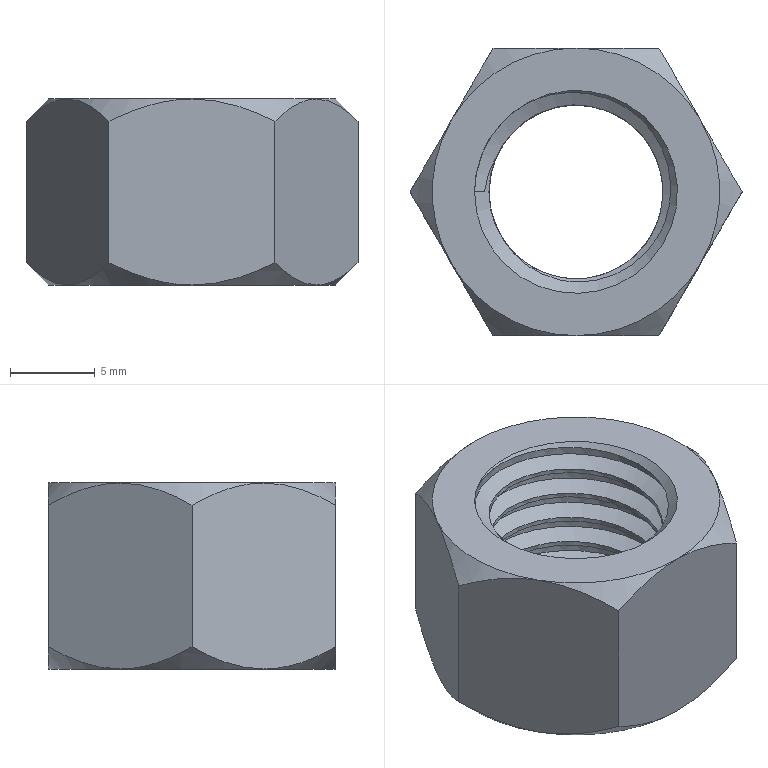Part | NX | features DATUM_CSYS 3, EXTRACT_DATUM_AXIS 2, EXTRACT_STRING 2, SKETCH 2, SWP104 2, EXTRUDE 1, HOLE PACKAGE 1, Instance Feature 1, Mirror Feature 1, SIMPLE HOLE 1, SYMBOLIC_THREAD 1, THREADS 1 | 1 solid | 28 faces | box 19.63 x 17 x 11 mm | volume 1644 mm3 | cone 14 | plane 10 | cylinder 2 | spline 2 | commonest cylinder face diameters 10.3 x1 12 x1